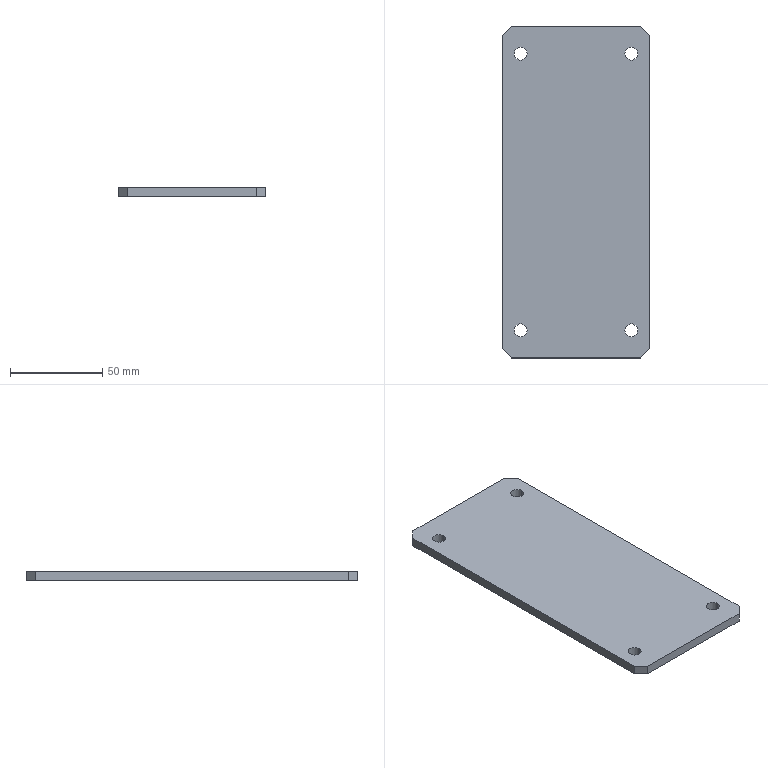Part | SolidWorks | features Chamfer 1, Extrusion 1, ICE 1 | 1 solid | 18 faces | box 80 x 180 x 5 mm | volume 70980 mm3 | plane 10 | cylinder 8 | commonest cylinder face diameters 7 x8
STEP:
#1=CARTESIAN_POINT('',(26.5,75.,0.));
#2=VERTEX_POINT('',#1);
#3=CARTESIAN_POINT('',(33.5,75.,0.));
#4=VERTEX_POINT('',#3);
#5=CARTESIAN_POINT('',(30.,75.,0.));
#6=DIRECTION('',(0.,0.,1.));
#7=DIRECTION('',(1.,0.,0.));
#8=AXIS2_PLACEMENT_3D('',#5,#6,#7);
#9=CIRCLE('',#8,3.5);
#10=EDGE_CURVE('',#2,#4,#9,.T.);
#11=ORIENTED_EDGE('',*,*,#10,.F.);
#12=CARTESIAN_POINT('',(26.5,75.,5.));
#13=VERTEX_POINT('',#12);
#14=CARTESIAN_POINT('',(26.5,75.,0.));
#15=DIRECTION('',(0.,0.,1.));
#16=VECTOR('',#15,1000.);
#17=LINE('',#14,#16);
#18=EDGE_CURVE('',#2,#13,#17,.T.);
#19=ORIENTED_EDGE('',*,*,#18,.T.);
#20=CARTESIAN_POINT('',(33.5,75.,5.));
#21=VERTEX_POINT('',#20);
#22=CARTESIAN_POINT('',(30.,75.,5.));
#23=DIRECTION('',(0.,0.,1.));
#24=DIRECTION('',(1.,0.,0.));
#25=AXIS2_PLACEMENT_3D('',#22,#23,#24);
#26=CIRCLE('',#25,3.5);
#27=EDGE_CURVE('',#13,#21,#26,.T.);
#28=ORIENTED_EDGE('',*,*,#27,.T.);
#29=CARTESIAN_POINT('',(33.5,75.,0.));
#30=DIRECTION('',(0.,0.,1.));
#31=VECTOR('',#30,1000.);
#32=LINE('',#29,#31);
#33=EDGE_CURVE('',#4,#21,#32,.T.);
#34=ORIENTED_EDGE('',*,*,#33,.F.);
#35=EDGE_LOOP('',(#11,#19,#28,#34));
#36=FACE_OUTER_BOUND('',#35,.T.);
#37=CARTESIAN_POINT('',(30.,75.,0.));
#38=DIRECTION('',(0.,0.,1.));
#39=DIRECTION('',(1.,0.,0.));
#40=AXIS2_PLACEMENT_3D('',#37,#38,#39);
#41=CYLINDRICAL_SURFACE('',#40,3.5);
#42=ADVANCED_FACE('',(#36),#41,.F.);
#43=CARTESIAN_POINT('',(-33.5,-75.,0.));
#44=VERTEX_POINT('',#43);
#45=CARTESIAN_POINT('',(-26.5,-75.,0.));
#46=VERTEX_POINT('',#45);
#47=CARTESIAN_POINT('',(-30.,-75.,0.));
#48=DIRECTION('',(0.,0.,1.));
#49=DIRECTION('',(1.,0.,0.));
#50=AXIS2_PLACEMENT_3D('',#47,#48,#49);
#51=CIRCLE('',#50,3.5);
#52=EDGE_CURVE('',#44,#46,#51,.T.);
#53=ORIENTED_EDGE('',*,*,#52,.F.);
#54=CARTESIAN_POINT('',(-33.5,-75.,5.));
#55=VERTEX_POINT('',#54);
#56=CARTESIAN_POINT('',(-33.5,-75.,0.));
#57=DIRECTION('',(0.,0.,1.));
#58=VECTOR('',#57,1000.);
#59=LINE('',#56,#58);
#60=EDGE_CURVE('',#44,#55,#59,.T.);
#61=ORIENTED_EDGE('',*,*,#60,.T.);
#62=CARTESIAN_POINT('',(-26.5,-75.,5.));
#63=VERTEX_POINT('',#62);
#64=CARTESIAN_POINT('',(-30.,-75.,5.));
#65=DIRECTION('',(0.,0.,1.));
#66=DIRECTION('',(1.,0.,0.));
#67=AXIS2_PLACEMENT_3D('',#64,#65,#66);
#68=CIRCLE('',#67,3.5);
#69=EDGE_CURVE('',#55,#63,#68,.T.);
#70=ORIENTED_EDGE('',*,*,#69,.T.);
#71=CARTESIAN_POINT('',(-26.5,-75.,0.));
#72=DIRECTION('',(0.,0.,1.));
#73=VECTOR('',#72,1000.);
#74=LINE('',#71,#73);
#75=EDGE_CURVE('',#46,#63,#74,.T.);
#76=ORIENTED_EDGE('',*,*,#75,.F.);
#77=EDGE_LOOP('',(#53,#61,#70,#76));
#78=FACE_OUTER_BOUND('',#77,.T.);
#79=CARTESIAN_POINT('',(-30.,-75.,0.));
#80=DIRECTION('',(0.,0.,1.));
#81=DIRECTION('',(1.,0.,0.));
#82=AXIS2_PLACEMENT_3D('',#79,#80,#81);
#83=CYLINDRICAL_SURFACE('',#82,3.5);
#84=ADVANCED_FACE('',(#78),#83,.F.);
#85=CARTESIAN_POINT('',(26.5,-75.,0.));
#86=VERTEX_POINT('',#85);
#87=CARTESIAN_POINT('',(33.5,-75.,0.));
#88=VERTEX_POINT('',#87);
#89=CARTESIAN_POINT('',(30.,-75.,0.));
#90=DIRECTION('',(0.,0.,1.));
#91=DIRECTION('',(1.,0.,0.));
#92=AXIS2_PLACEMENT_3D('',#89,#90,#91);
#93=CIRCLE('',#92,3.5);
#94=EDGE_CURVE('',#86,#88,#93,.T.);
#95=ORIENTED_EDGE('',*,*,#94,.F.);
#96=CARTESIAN_POINT('',(26.5,-75.,5.));
#97=VERTEX_POINT('',#96);
#98=CARTESIAN_POINT('',(26.5,-75.,0.));
#99=DIRECTION('',(0.,0.,1.));
#100=VECTOR('',#99,1000.);
#101=LINE('',#98,#100);
#102=EDGE_CURVE('',#86,#97,#101,.T.);
#103=ORIENTED_EDGE('',*,*,#102,.T.);
#104=CARTESIAN_POINT('',(33.5,-75.,5.));
#105=VERTEX_POINT('',#104);
#106=CARTESIAN_POINT('',(30.,-75.,5.));
#107=DIRECTION('',(0.,0.,1.));
#108=DIRECTION('',(1.,0.,0.));
#109=AXIS2_PLACEMENT_3D('',#106,#107,#108);
#110=CIRCLE('',#109,3.5);
#111=EDGE_CURVE('',#97,#105,#110,.T.);
#112=ORIENTED_EDGE('',*,*,#111,.T.);
#113=CARTESIAN_POINT('',(33.5,-75.,0.));
#114=DIRECTION('',(0.,0.,1.));
#115=VECTOR('',#114,1000.);
#116=LINE('',#113,#115);
#117=EDGE_CURVE('',#88,#105,#116,.T.);
#118=ORIENTED_EDGE('',*,*,#117,.F.);
#119=EDGE_LOOP('',(#95,#103,#112,#118));
#120=FACE_OUTER_BOUND('',#119,.T.);
#121=CARTESIAN_POINT('',(30.,-75.,0.));
#122=DIRECTION('',(0.,0.,1.));
#123=DIRECTION('',(1.,0.,0.));
#124=AXIS2_PLACEMENT_3D('',#121,#122,#123);
#125=CYLINDRICAL_SURFACE('',#124,3.5);
#126=ADVANCED_FACE('',(#120),#125,.F.);
#127=CARTESIAN_POINT('',(-33.5,75.,0.));
#128=VERTEX_POINT('',#127);
#129=CARTESIAN_POINT('',(-26.5,75.,0.));
#130=VERTEX_POINT('',#129);
#131=CARTESIAN_POINT('',(-30.,75.,0.));
#132=DIRECTION('',(0.,0.,1.));
#133=DIRECTION('',(1.,0.,0.));
#134=AXIS2_PLACEMENT_3D('',#131,#132,#133);
#135=CIRCLE('',#134,3.5);
#136=EDGE_CURVE('',#128,#130,#135,.T.);
#137=ORIENTED_EDGE('',*,*,#136,.F.);
#138=CARTESIAN_POINT('',(-33.5,75.,5.));
#139=VERTEX_POINT('',#138);
#140=CARTESIAN_POINT('',(-33.5,75.,0.));
#141=DIRECTION('',(0.,0.,1.));
#142=VECTOR('',#141,1000.);
#143=LINE('',#140,#142);
#144=EDGE_CURVE('',#128,#139,#143,.T.);
#145=ORIENTED_EDGE('',*,*,#144,.T.);
#146=CARTESIAN_POINT('',(-26.5,75.,5.));
#147=VERTEX_POINT('',#146);
#148=CARTESIAN_POINT('',(-30.,75.,5.));
#149=DIRECTION('',(0.,0.,1.));
#150=DIRECTION('',(1.,0.,0.));
#151=AXIS2_PLACEMENT_3D('',#148,#149,#150);
#152=CIRCLE('',#151,3.5);
#153=EDGE_CURVE('',#139,#147,#152,.T.);
#154=ORIENTED_EDGE('',*,*,#153,.T.);
#155=CARTESIAN_POINT('',(-26.5,75.,0.));
#156=DIRECTION('',(0.,0.,1.));
#157=VECTOR('',#156,1000.);
#158=LINE('',#155,#157);
#159=EDGE_CURVE('',#130,#147,#158,.T.);
#160=ORIENTED_EDGE('',*,*,#159,.F.);
#161=EDGE_LOOP('',(#137,#145,#154,#160));
#162=FACE_OUTER_BOUND('',#161,.T.);
#163=CARTESIAN_POINT('',(-30.,75.,0.));
#164=DIRECTION('',(0.,0.,1.));
#165=DIRECTION('',(1.,0.,0.));
#166=AXIS2_PLACEMENT_3D('',#163,#164,#165);
#167=CYLINDRICAL_SURFACE('',#166,3.5);
#168=ADVANCED_FACE('',(#162),#167,.F.);
#169=CARTESIAN_POINT('',(40.,-85.,5.));
#170=VERTEX_POINT('',#169);
#171=CARTESIAN_POINT('',(40.,85.,5.));
#172=VERTEX_POINT('',#171);
#173=CARTESIAN_POINT('',(40.,90.,5.));
#174=DIRECTION('',(0.,1.,0.));
#175=VECTOR('',#174,1000.);
#176=LINE('',#173,#175);
#177=EDGE_CURVE('',#170,#172,#176,.T.);
#178=ORIENTED_EDGE('',*,*,#177,.F.);
#179=CARTESIAN_POINT('',(40.,-85.,0.));
#180=VERTEX_POINT('',#179);
#181=CARTESIAN_POINT('',(40.,-85.,5.));
#182=DIRECTION('',(0.,0.,-1.));
#183=VECTOR('',#182,1000.);
#184=LINE('',#181,#183);
#185=EDGE_CURVE('',#170,#180,#184,.T.);
#186=ORIENTED_EDGE('',*,*,#185,.T.);
#187=CARTESIAN_POINT('',(40.,85.,0.));
#188=VERTEX_POINT('',#187);
#189=CARTESIAN_POINT('',(40.,90.,0.));
#190=DIRECTION('',(0.,1.,0.));
#191=VECTOR('',#190,1000.);
#192=LINE('',#189,#191);
#193=EDGE_CURVE('',#180,#188,#192,.T.);
#194=ORIENTED_EDGE('',*,*,#193,.T.);
#195=CARTESIAN_POINT('',(40.,85.,5.));
#196=DIRECTION('',(0.,0.,1.));
#197=VECTOR('',#196,1000.);
#198=LINE('',#195,#197);
#199=EDGE_CURVE('',#188,#172,#198,.T.);
#200=ORIENTED_EDGE('',*,*,#199,.T.);
#201=EDGE_LOOP('',(#178,#186,#194,#200));
#202=FACE_OUTER_BOUND('',#201,.T.);
#203=CARTESIAN_POINT('',(40.,90.,5.));
#204=DIRECTION('',(-1.,0.,0.));
#205=DIRECTION('',(0.,-1.,0.));
#206=AXIS2_PLACEMENT_3D('',#203,#204,#205);
#207=PLANE('',#206);
#208=ADVANCED_FACE('',(#202),#207,.F.);
#209=CARTESIAN_POINT('',(35.,90.,5.));
#210=VERTEX_POINT('',#209);
#211=CARTESIAN_POINT('',(-35.,90.,5.));
#212=VERTEX_POINT('',#211);
#213=CARTESIAN_POINT('',(-40.,90.,5.));
#214=DIRECTION('',(-1.,0.,0.));
#215=VECTOR('',#214,1000.);
#216=LINE('',#213,#215);
#217=EDGE_CURVE('',#210,#212,#216,.T.);
#218=ORIENTED_EDGE('',*,*,#217,.F.);
#219=CARTESIAN_POINT('',(35.,90.,0.));
#220=VERTEX_POINT('',#219);
#221=CARTESIAN_POINT('',(35.,90.,5.));
#222=DIRECTION('',(0.,0.,-1.));
#223=VECTOR('',#222,1000.);
#224=LINE('',#221,#223);
#225=EDGE_CURVE('',#210,#220,#224,.T.);
#226=ORIENTED_EDGE('',*,*,#225,.T.);
#227=CARTESIAN_POINT('',(-35.,90.,0.));
#228=VERTEX_POINT('',#227);
#229=CARTESIAN_POINT('',(-40.,90.,0.));
#230=DIRECTION('',(-1.,0.,0.));
#231=VECTOR('',#230,1000.);
#232=LINE('',#229,#231);
#233=EDGE_CURVE('',#220,#228,#232,.T.);
#234=ORIENTED_EDGE('',*,*,#233,.T.);
#235=CARTESIAN_POINT('',(-35.,90.,5.));
#236=DIRECTION('',(0.,0.,1.));
#237=VECTOR('',#236,1000.);
#238=LINE('',#235,#237);
#239=EDGE_CURVE('',#228,#212,#238,.T.);
#240=ORIENTED_EDGE('',*,*,#239,.T.);
#241=EDGE_LOOP('',(#218,#226,#234,#240));
#242=FACE_OUTER_BOUND('',#241,.T.);
#243=CARTESIAN_POINT('',(-40.,90.,5.));
#244=DIRECTION('',(0.,-1.,0.));
#245=DIRECTION('',(0.,0.,-1.));
#246=AXIS2_PLACEMENT_3D('',#243,#244,#245);
#247=PLANE('',#246);
#248=ADVANCED_FACE('',(#242),#247,.F.);
#249=CARTESIAN_POINT('',(-40.,85.,0.));
#250=VERTEX_POINT('',#249);
#251=CARTESIAN_POINT('',(-40.,-85.,0.));
#252=VERTEX_POINT('',#251);
#253=CARTESIAN_POINT('',(-40.,90.,0.));
#254=DIRECTION('',(0.,-1.,0.));
#255=VECTOR('',#254,1000.);
#256=LINE('',#253,#255);
#257=EDGE_CURVE('',#250,#252,#256,.T.);
#258=ORIENTED_EDGE('',*,*,#257,.T.);
#259=CARTESIAN_POINT('',(-40.,-85.,5.));
#260=VERTEX_POINT('',#259);
#261=CARTESIAN_POINT('',(-40.,-85.,5.));
#262=DIRECTION('',(0.,0.,1.));
#263=VECTOR('',#262,1000.);
#264=LINE('',#261,#263);
#265=EDGE_CURVE('',#252,#260,#264,.T.);
#266=ORIENTED_EDGE('',*,*,#265,.T.);
#267=CARTESIAN_POINT('',(-40.,85.,5.));
#268=VERTEX_POINT('',#267);
#269=CARTESIAN_POINT('',(-40.,90.,5.));
#270=DIRECTION('',(0.,-1.,0.));
#271=VECTOR('',#270,1000.);
#272=LINE('',#269,#271);
#273=EDGE_CURVE('',#268,#260,#272,.T.);
#274=ORIENTED_EDGE('',*,*,#273,.F.);
#275=CARTESIAN_POINT('',(-40.,85.,5.));
#276=DIRECTION('',(0.,0.,-1.));
#277=VECTOR('',#276,1000.);
#278=LINE('',#275,#277);
#279=EDGE_CURVE('',#268,#250,#278,.T.);
#280=ORIENTED_EDGE('',*,*,#279,.T.);
#281=EDGE_LOOP('',(#258,#266,#274,#280));
#282=FACE_OUTER_BOUND('',#281,.T.);
#283=CARTESIAN_POINT('',(-40.,90.,5.));
#284=DIRECTION('',(1.,0.,0.));
#285=DIRECTION('',(0.,1.,0.));
#286=AXIS2_PLACEMENT_3D('',#283,#284,#285);
#287=PLANE('',#286);
#288=ADVANCED_FACE('',(#282),#287,.F.);
#289=CARTESIAN_POINT('',(-35.,-90.,5.));
#290=VERTEX_POINT('',#289);
#291=CARTESIAN_POINT('',(35.,-90.,5.));
#292=VERTEX_POINT('',#291);
#293=CARTESIAN_POINT('',(-40.,-90.,5.));
#294=DIRECTION('',(1.,0.,0.));
#295=VECTOR('',#294,1000.);
#296=LINE('',#293,#295);
#297=EDGE_CURVE('',#290,#292,#296,.T.);
#298=ORIENTED_EDGE('',*,*,#297,.F.);
#299=CARTESIAN_POINT('',(-35.,-90.,0.));
#300=VERTEX_POINT('',#299);
#301=CARTESIAN_POINT('',(-35.,-90.,5.));
#302=DIRECTION('',(0.,0.,-1.));
#303=VECTOR('',#302,1000.);
#304=LINE('',#301,#303);
#305=EDGE_CURVE('',#290,#300,#304,.T.);
#306=ORIENTED_EDGE('',*,*,#305,.T.);
#307=CARTESIAN_POINT('',(35.,-90.,0.));
#308=VERTEX_POINT('',#307);
#309=CARTESIAN_POINT('',(-40.,-90.,0.));
#310=DIRECTION('',(1.,0.,0.));
#311=VECTOR('',#310,1000.);
#312=LINE('',#309,#311);
#313=EDGE_CURVE('',#300,#308,#312,.T.);
#314=ORIENTED_EDGE('',*,*,#313,.T.);
#315=CARTESIAN_POINT('',(35.,-90.,5.));
#316=DIRECTION('',(0.,0.,1.));
#317=VECTOR('',#316,1000.);
#318=LINE('',#315,#317);
#319=EDGE_CURVE('',#308,#292,#318,.T.);
#320=ORIENTED_EDGE('',*,*,#319,.T.);
#321=EDGE_LOOP('',(#298,#306,#314,#320));
#322=FACE_OUTER_BOUND('',#321,.T.);
#323=CARTESIAN_POINT('',(-40.,-90.,5.));
#324=DIRECTION('',(0.,1.,0.));
#325=DIRECTION('',(0.,0.,1.));
#326=AXIS2_PLACEMENT_3D('',#323,#324,#325);
#327=PLANE('',#326);
#328=ADVANCED_FACE('',(#322),#327,.F.);
#329=CARTESIAN_POINT('',(30.,75.,5.));
#330=DIRECTION('',(0.,0.,1.));
#331=DIRECTION('',(1.,0.,0.));
#332=AXIS2_PLACEMENT_3D('',#329,#330,#331);
#333=CIRCLE('',#332,3.5);
#334=EDGE_CURVE('',#21,#13,#333,.T.);
#335=ORIENTED_EDGE('',*,*,#334,.F.);
#336=ORIENTED_EDGE('',*,*,#27,.F.);
#337=EDGE_LOOP('',(#335,#336));
#338=FACE_BOUND('',#337,.T.);
#339=CARTESIAN_POINT('',(-30.,-75.,5.));
#340=DIRECTION('',(0.,0.,1.));
#341=DIRECTION('',(1.,0.,0.));
#342=AXIS2_PLACEMENT_3D('',#339,#340,#341);
#343=CIRCLE('',#342,3.5);
#344=EDGE_CURVE('',#63,#55,#343,.T.);
#345=ORIENTED_EDGE('',*,*,#344,.F.);
#346=ORIENTED_EDGE('',*,*,#69,.F.);
#347=EDGE_LOOP('',(#345,#346));
#348=FACE_BOUND('',#347,.T.);
#349=CARTESIAN_POINT('',(30.,-75.,5.));
#350=DIRECTION('',(0.,0.,1.));
#351=DIRECTION('',(1.,0.,0.));
#352=AXIS2_PLACEMENT_3D('',#349,#350,#351);
#353=CIRCLE('',#352,3.5);
#354=EDGE_CURVE('',#105,#97,#353,.T.);
#355=ORIENTED_EDGE('',*,*,#354,.F.);
#356=ORIENTED_EDGE('',*,*,#111,.F.);
#357=EDGE_LOOP('',(#355,#356));
#358=FACE_BOUND('',#357,.T.);
#359=CARTESIAN_POINT('',(-30.,75.,5.));
#360=DIRECTION('',(0.,0.,1.));
#361=DIRECTION('',(1.,0.,0.));
#362=AXIS2_PLACEMENT_3D('',#359,#360,#361);
#363=CIRCLE('',#362,3.5);
#364=EDGE_CURVE('',#147,#139,#363,.T.);
#365=ORIENTED_EDGE('',*,*,#364,.F.);
#366=ORIENTED_EDGE('',*,*,#153,.F.);
#367=EDGE_LOOP('',(#365,#366));
#368=FACE_BOUND('',#367,.T.);
#369=ORIENTED_EDGE('',*,*,#273,.T.);
#370=CARTESIAN_POINT('',(-62.5,-62.5,5.));
#371=DIRECTION('',(0.7071,-0.7071,0.));
#372=VECTOR('',#371,1000.);
#373=LINE('',#370,#372);
#374=EDGE_CURVE('',#260,#290,#373,.T.);
#375=ORIENTED_EDGE('',*,*,#374,.T.);
#376=ORIENTED_EDGE('',*,*,#297,.T.);
#377=CARTESIAN_POINT('',(62.5,-62.5,5.));
#378=DIRECTION('',(0.7071,0.7071,0.));
#379=VECTOR('',#378,1000.);
#380=LINE('',#377,#379);
#381=EDGE_CURVE('',#292,#170,#380,.T.);
#382=ORIENTED_EDGE('',*,*,#381,.T.);
#383=ORIENTED_EDGE('',*,*,#177,.T.);
#384=CARTESIAN_POINT('',(62.5,62.5,5.));
#385=DIRECTION('',(-0.7071,0.7071,0.));
#386=VECTOR('',#385,1000.);
#387=LINE('',#384,#386);
#388=EDGE_CURVE('',#172,#210,#387,.T.);
#389=ORIENTED_EDGE('',*,*,#388,.T.);
#390=ORIENTED_EDGE('',*,*,#217,.T.);
#391=CARTESIAN_POINT('',(-62.5,62.5,5.));
#392=DIRECTION('',(-0.7071,-0.7071,0.));
#393=VECTOR('',#392,1000.);
#394=LINE('',#391,#393);
#395=EDGE_CURVE('',#212,#268,#394,.T.);
#396=ORIENTED_EDGE('',*,*,#395,.T.);
#397=EDGE_LOOP('',(#369,#375,#376,#382,#383,#389,#390,#396));
#398=FACE_OUTER_BOUND('',#397,.T.);
#399=CARTESIAN_POINT('',(0.,0.,5.));
#400=DIRECTION('',(0.,0.,1.));
#401=DIRECTION('',(1.,0.,0.));
#402=AXIS2_PLACEMENT_3D('',#399,#400,#401);
#403=PLANE('',#402);
#404=ADVANCED_FACE('',(#338,#348,#358,#368,#398),#403,.T.);
#405=CARTESIAN_POINT('',(30.,75.,0.));
#406=DIRECTION('',(0.,0.,1.));
#407=DIRECTION('',(1.,0.,0.));
#408=AXIS2_PLACEMENT_3D('',#405,#406,#407);
#409=CIRCLE('',#408,3.5);
#410=EDGE_CURVE('',#4,#2,#409,.T.);
#411=ORIENTED_EDGE('',*,*,#410,.T.);
#412=ORIENTED_EDGE('',*,*,#10,.T.);
#413=EDGE_LOOP('',(#411,#412));
#414=FACE_BOUND('',#413,.T.);
#415=CARTESIAN_POINT('',(-30.,-75.,0.));
#416=DIRECTION('',(0.,0.,1.));
#417=DIRECTION('',(1.,0.,0.));
#418=AXIS2_PLACEMENT_3D('',#415,#416,#417);
#419=CIRCLE('',#418,3.5);
#420=EDGE_CURVE('',#46,#44,#419,.T.);
#421=ORIENTED_EDGE('',*,*,#420,.T.);
#422=ORIENTED_EDGE('',*,*,#52,.T.);
#423=EDGE_LOOP('',(#421,#422));
#424=FACE_BOUND('',#423,.T.);
#425=CARTESIAN_POINT('',(30.,-75.,0.));
#426=DIRECTION('',(0.,0.,1.));
#427=DIRECTION('',(1.,0.,0.));
#428=AXIS2_PLACEMENT_3D('',#425,#426,#427);
#429=CIRCLE('',#428,3.5);
#430=EDGE_CURVE('',#88,#86,#429,.T.);
#431=ORIENTED_EDGE('',*,*,#430,.T.);
#432=ORIENTED_EDGE('',*,*,#94,.T.);
#433=EDGE_LOOP('',(#431,#432));
#434=FACE_BOUND('',#433,.T.);
#435=CARTESIAN_POINT('',(-30.,75.,0.));
#436=DIRECTION('',(0.,0.,1.));
#437=DIRECTION('',(1.,0.,0.));
#438=AXIS2_PLACEMENT_3D('',#435,#436,#437);
#439=CIRCLE('',#438,3.5);
#440=EDGE_CURVE('',#130,#128,#439,.T.);
#441=ORIENTED_EDGE('',*,*,#440,.T.);
#442=ORIENTED_EDGE('',*,*,#136,.T.);
#443=EDGE_LOOP('',(#441,#442));
#444=FACE_BOUND('',#443,.T.);
#445=ORIENTED_EDGE('',*,*,#313,.F.);
#446=CARTESIAN_POINT('',(-35.,-90.,0.));
#447=DIRECTION('',(-0.7071,0.7071,0.));
#448=VECTOR('',#447,1000.);
#449=LINE('',#446,#448);
#450=EDGE_CURVE('',#300,#252,#449,.T.);
#451=ORIENTED_EDGE('',*,*,#450,.T.);
#452=ORIENTED_EDGE('',*,*,#257,.F.);
#453=CARTESIAN_POINT('',(-40.,85.,0.));
#454=DIRECTION('',(0.7071,0.7071,0.));
#455=VECTOR('',#454,1000.);
#456=LINE('',#453,#455);
#457=EDGE_CURVE('',#250,#228,#456,.T.);
#458=ORIENTED_EDGE('',*,*,#457,.T.);
#459=ORIENTED_EDGE('',*,*,#233,.F.);
#460=CARTESIAN_POINT('',(35.,90.,0.));
#461=DIRECTION('',(0.7071,-0.7071,0.));
#462=VECTOR('',#461,1000.);
#463=LINE('',#460,#462);
#464=EDGE_CURVE('',#220,#188,#463,.T.);
#465=ORIENTED_EDGE('',*,*,#464,.T.);
#466=ORIENTED_EDGE('',*,*,#193,.F.);
#467=CARTESIAN_POINT('',(40.,-85.,0.));
#468=DIRECTION('',(-0.7071,-0.7071,0.));
#469=VECTOR('',#468,1000.);
#470=LINE('',#467,#469);
#471=EDGE_CURVE('',#180,#308,#470,.T.);
#472=ORIENTED_EDGE('',*,*,#471,.T.);
#473=EDGE_LOOP('',(#445,#451,#452,#458,#459,#465,#466,#472));
#474=FACE_OUTER_BOUND('',#473,.T.);
#475=CARTESIAN_POINT('',(0.,0.,0.));
#476=DIRECTION('',(0.,0.,1.));
#477=DIRECTION('',(1.,0.,0.));
#478=AXIS2_PLACEMENT_3D('',#475,#476,#477);
#479=PLANE('',#478);
#480=ADVANCED_FACE('',(#414,#424,#434,#444,#474),#479,.F.);
#481=ORIENTED_EDGE('',*,*,#374,.F.);
#482=ORIENTED_EDGE('',*,*,#265,.F.);
#483=ORIENTED_EDGE('',*,*,#450,.F.);
#484=ORIENTED_EDGE('',*,*,#305,.F.);
#485=EDGE_LOOP('',(#481,#482,#483,#484));
#486=FACE_OUTER_BOUND('',#485,.T.);
#487=CARTESIAN_POINT('',(-35.,-90.,5.));
#488=DIRECTION('',(0.7071,0.7071,0.));
#489=DIRECTION('',(0.,0.,-1.));
#490=AXIS2_PLACEMENT_3D('',#487,#488,#489);
#491=PLANE('',#490);
#492=ADVANCED_FACE('',(#486),#491,.F.);
#493=ORIENTED_EDGE('',*,*,#381,.F.);
#494=ORIENTED_EDGE('',*,*,#319,.F.);
#495=ORIENTED_EDGE('',*,*,#471,.F.);
#496=ORIENTED_EDGE('',*,*,#185,.F.);
#497=EDGE_LOOP('',(#493,#494,#495,#496));
#498=FACE_OUTER_BOUND('',#497,.T.);
#499=CARTESIAN_POINT('',(40.,-85.,5.));
#500=DIRECTION('',(-0.7071,0.7071,0.));
#501=DIRECTION('',(0.,0.,-1.));
#502=AXIS2_PLACEMENT_3D('',#499,#500,#501);
#503=PLANE('',#502);
#504=ADVANCED_FACE('',(#498),#503,.F.);
#505=ORIENTED_EDGE('',*,*,#388,.F.);
#506=ORIENTED_EDGE('',*,*,#199,.F.);
#507=ORIENTED_EDGE('',*,*,#464,.F.);
#508=ORIENTED_EDGE('',*,*,#225,.F.);
#509=EDGE_LOOP('',(#505,#506,#507,#508));
#510=FACE_OUTER_BOUND('',#509,.T.);
#511=CARTESIAN_POINT('',(35.,90.,5.));
#512=DIRECTION('',(-0.7071,-0.7071,0.));
#513=DIRECTION('',(0.,0.,-1.));
#514=AXIS2_PLACEMENT_3D('',#511,#512,#513);
#515=PLANE('',#514);
#516=ADVANCED_FACE('',(#510),#515,.F.);
#517=ORIENTED_EDGE('',*,*,#395,.F.);
#518=ORIENTED_EDGE('',*,*,#239,.F.);
#519=ORIENTED_EDGE('',*,*,#457,.F.);
#520=ORIENTED_EDGE('',*,*,#279,.F.);
#521=EDGE_LOOP('',(#517,#518,#519,#520));
#522=FACE_OUTER_BOUND('',#521,.T.);
#523=CARTESIAN_POINT('',(-40.,85.,5.));
#524=DIRECTION('',(0.7071,-0.7071,0.));
#525=DIRECTION('',(0.,0.,-1.));
#526=AXIS2_PLACEMENT_3D('',#523,#524,#525);
#527=PLANE('',#526);
#528=ADVANCED_FACE('',(#522),#527,.F.);
#529=ORIENTED_EDGE('',*,*,#144,.F.);
#530=ORIENTED_EDGE('',*,*,#440,.F.);
#531=ORIENTED_EDGE('',*,*,#159,.T.);
#532=ORIENTED_EDGE('',*,*,#364,.T.);
#533=EDGE_LOOP('',(#529,#530,#531,#532));
#534=FACE_OUTER_BOUND('',#533,.T.);
#535=CARTESIAN_POINT('',(-30.,75.,0.));
#536=DIRECTION('',(0.,0.,1.));
#537=DIRECTION('',(1.,0.,0.));
#538=AXIS2_PLACEMENT_3D('',#535,#536,#537);
#539=CYLINDRICAL_SURFACE('',#538,3.5);
#540=ADVANCED_FACE('',(#534),#539,.F.);
#541=ORIENTED_EDGE('',*,*,#102,.F.);
#542=ORIENTED_EDGE('',*,*,#430,.F.);
#543=ORIENTED_EDGE('',*,*,#117,.T.);
#544=ORIENTED_EDGE('',*,*,#354,.T.);
#545=EDGE_LOOP('',(#541,#542,#543,#544));
#546=FACE_OUTER_BOUND('',#545,.T.);
#547=CARTESIAN_POINT('',(30.,-75.,0.));
#548=DIRECTION('',(0.,0.,1.));
#549=DIRECTION('',(1.,0.,0.));
#550=AXIS2_PLACEMENT_3D('',#547,#548,#549);
#551=CYLINDRICAL_SURFACE('',#550,3.5);
#552=ADVANCED_FACE('',(#546),#551,.F.);
#553=ORIENTED_EDGE('',*,*,#60,.F.);
#554=ORIENTED_EDGE('',*,*,#420,.F.);
#555=ORIENTED_EDGE('',*,*,#75,.T.);
#556=ORIENTED_EDGE('',*,*,#344,.T.);
#557=EDGE_LOOP('',(#553,#554,#555,#556));
#558=FACE_OUTER_BOUND('',#557,.T.);
#559=CARTESIAN_POINT('',(-30.,-75.,0.));
#560=DIRECTION('',(0.,0.,1.));
#561=DIRECTION('',(1.,0.,0.));
#562=AXIS2_PLACEMENT_3D('',#559,#560,#561);
#563=CYLINDRICAL_SURFACE('',#562,3.5);
#564=ADVANCED_FACE('',(#558),#563,.F.);
#565=ORIENTED_EDGE('',*,*,#18,.F.);
#566=ORIENTED_EDGE('',*,*,#410,.F.);
#567=ORIENTED_EDGE('',*,*,#33,.T.);
#568=ORIENTED_EDGE('',*,*,#334,.T.);
#569=EDGE_LOOP('',(#565,#566,#567,#568));
#570=FACE_OUTER_BOUND('',#569,.T.);
#571=CARTESIAN_POINT('',(30.,75.,0.));
#572=DIRECTION('',(0.,0.,1.));
#573=DIRECTION('',(1.,0.,0.));
#574=AXIS2_PLACEMENT_3D('',#571,#572,#573);
#575=CYLINDRICAL_SURFACE('',#574,3.5);
#576=ADVANCED_FACE('',(#570),#575,.F.);
#577=CLOSED_SHELL('',(#42,#84,#126,#168,#208,#248,#288,#328,#404,#480,#492,#504,#516,#528,#540,#552,#564,#576));
#578=MANIFOLD_SOLID_BREP('',#577);
#579=CARTESIAN_POINT('',(0.,0.,0.));
#580=DIRECTION('',(0.,0.,1.));
#581=DIRECTION('',(1.,0.,0.));
#582=AXIS2_PLACEMENT_3D('',#579,#580,#581);
#583=(LENGTH_UNIT()NAMED_UNIT(*)SI_UNIT(.MILLI.,.METRE.));
#584=UNCERTAINTY_MEASURE_WITH_UNIT(LENGTH_MEASURE(0.00001),#583,'','');
#585=(NAMED_UNIT(*)PLANE_ANGLE_UNIT()SI_UNIT($,.RADIAN.));
#586=(NAMED_UNIT(*)SI_UNIT($,.STERADIAN.)SOLID_ANGLE_UNIT());
#587=(GEOMETRIC_REPRESENTATION_CONTEXT(3)GLOBAL_UNCERTAINTY_ASSIGNED_CONTEXT((#584))GLOBAL_UNIT_ASSIGNED_CONTEXT((#583,#585,#586))REPRESENTATION_CONTEXT('',''));
#588=ADVANCED_BREP_SHAPE_REPRESENTATION('',(#578,#582),#587);